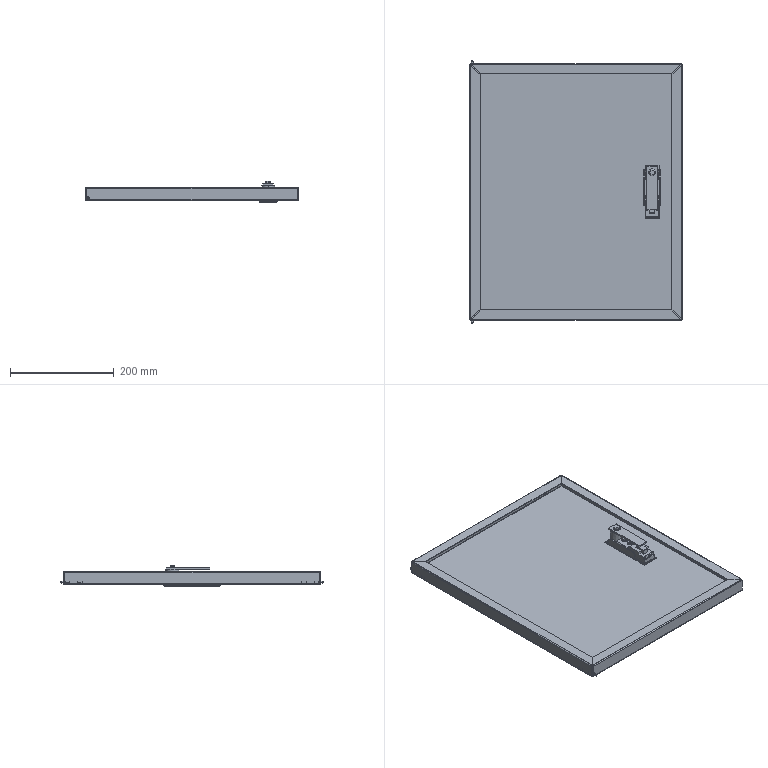Part | SolidWorks | 6 solids | 422 faces | box 411 x 509 x 42.5 mm | volume 486734 mm3 | plane 238 | cylinder 144 | spline 28 | cone 12 | commonest cylinder face diameters 4 x34 1 x17 2 x15 12 x8 8 x6 3 x5